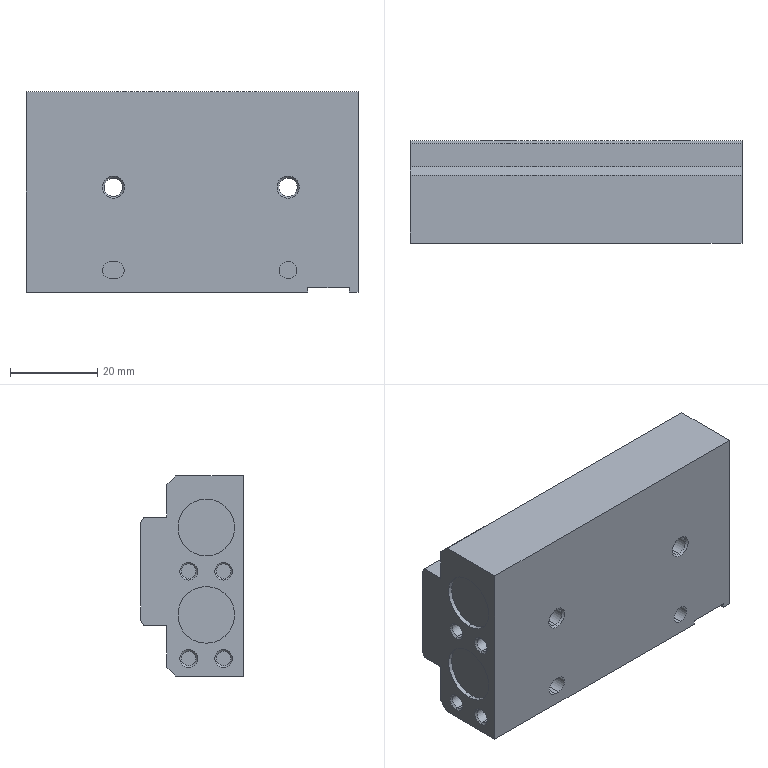Part | STEP file | 0246_Z_102_MXQ12L-30AS-A93_4 | 1 solid | 98 faces | box 76 x 23.5 x 45.8 mm | volume 60352 mm3 | cylinder 40 | plane 38 | cone 20 | commonest cylinder face diameters 3.3 x12 4.2 x8 4 x4 6 x4 8.5 x4 12 x4